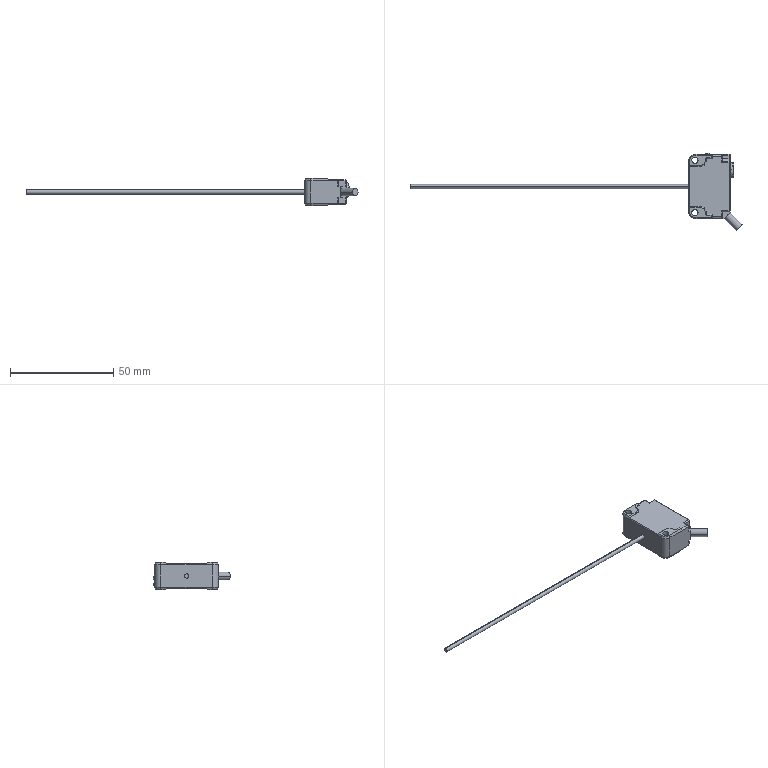Part | SolidWorks | features BaseBody 2 | 2 solids | 213 faces | box 160.77 x 37.32 x 13.1 mm | volume 7719 mm3 | plane 113 | cylinder 85 | cone 15 | commonest cylinder face diameters 0.3 x25 0.5 x22 2.5 x6 6 x6 0.2 x5 1 x4